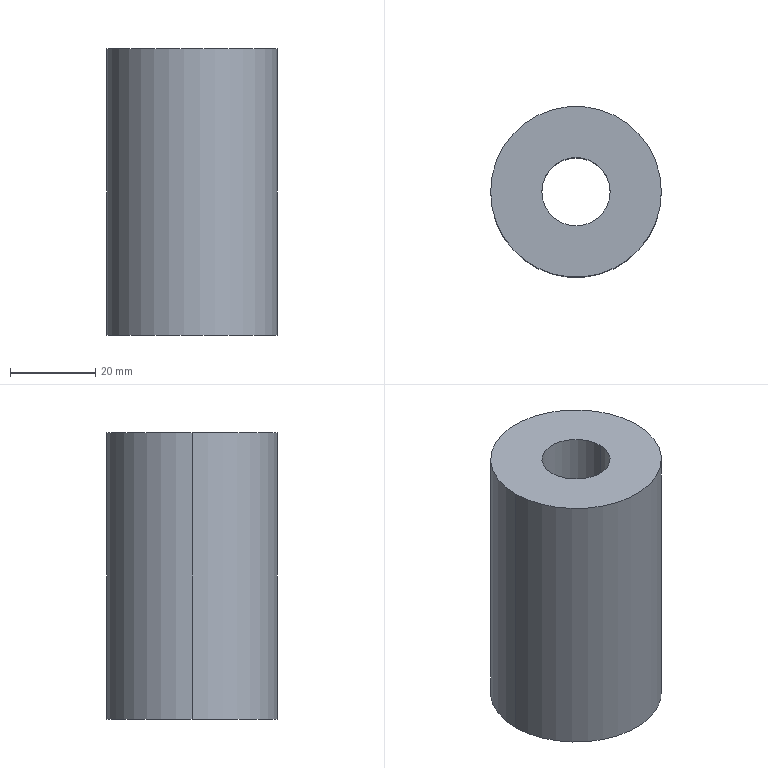Part | SolidWorks | features Extrusion 1, ICE 1 | 1 solid | 6 faces | box 40 x 40 x 67 mm | volume 70724 mm3 | cylinder 4 | plane 2 | commonest cylinder face diameters 16 x2 40 x2
STEP:
#1=CARTESIAN_POINT('',(-8.,0.,0.));
#2=VERTEX_POINT('',#1);
#3=CARTESIAN_POINT('',(8.,0.,0.));
#4=VERTEX_POINT('',#3);
#5=CARTESIAN_POINT('',(0.,0.,0.));
#6=DIRECTION('',(0.,0.,1.));
#7=DIRECTION('',(1.,0.,0.));
#8=AXIS2_PLACEMENT_3D('',#5,#6,#7);
#9=CIRCLE('',#8,8.);
#10=EDGE_CURVE('',#2,#4,#9,.T.);
#11=ORIENTED_EDGE('',*,*,#10,.F.);
#12=CARTESIAN_POINT('',(-8.,0.,67.));
#13=VERTEX_POINT('',#12);
#14=CARTESIAN_POINT('',(-8.,0.,-34.));
#15=DIRECTION('',(0.,0.,1.));
#16=VECTOR('',#15,1000.);
#17=LINE('',#14,#16);
#18=EDGE_CURVE('',#2,#13,#17,.T.);
#19=ORIENTED_EDGE('',*,*,#18,.T.);
#20=CARTESIAN_POINT('',(8.,0.,67.));
#21=VERTEX_POINT('',#20);
#22=CARTESIAN_POINT('',(0.,0.,67.));
#23=DIRECTION('',(0.,0.,1.));
#24=DIRECTION('',(1.,0.,0.));
#25=AXIS2_PLACEMENT_3D('',#22,#23,#24);
#26=CIRCLE('',#25,8.);
#27=EDGE_CURVE('',#13,#21,#26,.T.);
#28=ORIENTED_EDGE('',*,*,#27,.T.);
#29=CARTESIAN_POINT('',(8.,0.,-34.));
#30=DIRECTION('',(0.,0.,1.));
#31=VECTOR('',#30,1000.);
#32=LINE('',#29,#31);
#33=EDGE_CURVE('',#4,#21,#32,.T.);
#34=ORIENTED_EDGE('',*,*,#33,.F.);
#35=EDGE_LOOP('',(#11,#19,#28,#34));
#36=FACE_OUTER_BOUND('',#35,.T.);
#37=CARTESIAN_POINT('',(0.,0.,-34.));
#38=DIRECTION('',(0.,0.,1.));
#39=DIRECTION('',(1.,0.,0.));
#40=AXIS2_PLACEMENT_3D('',#37,#38,#39);
#41=CYLINDRICAL_SURFACE('',#40,8.);
#42=ADVANCED_FACE('',(#36),#41,.F.);
#43=CARTESIAN_POINT('',(20.,0.,67.));
#44=VERTEX_POINT('',#43);
#45=CARTESIAN_POINT('',(-20.,0.,67.));
#46=VERTEX_POINT('',#45);
#47=CARTESIAN_POINT('',(0.,0.,67.));
#48=DIRECTION('',(0.,0.,1.));
#49=DIRECTION('',(1.,0.,0.));
#50=AXIS2_PLACEMENT_3D('',#47,#48,#49);
#51=CIRCLE('',#50,20.);
#52=EDGE_CURVE('',#44,#46,#51,.T.);
#53=ORIENTED_EDGE('',*,*,#52,.F.);
#54=CARTESIAN_POINT('',(20.,0.,0.));
#55=VERTEX_POINT('',#54);
#56=CARTESIAN_POINT('',(20.,0.,67.));
#57=DIRECTION('',(0.,0.,-1.));
#58=VECTOR('',#57,1000.);
#59=LINE('',#56,#58);
#60=EDGE_CURVE('',#44,#55,#59,.T.);
#61=ORIENTED_EDGE('',*,*,#60,.T.);
#62=CARTESIAN_POINT('',(-20.,0.,0.));
#63=VERTEX_POINT('',#62);
#64=CARTESIAN_POINT('',(0.,0.,0.));
#65=DIRECTION('',(0.,0.,1.));
#66=DIRECTION('',(1.,0.,0.));
#67=AXIS2_PLACEMENT_3D('',#64,#65,#66);
#68=CIRCLE('',#67,20.);
#69=EDGE_CURVE('',#55,#63,#68,.T.);
#70=ORIENTED_EDGE('',*,*,#69,.T.);
#71=CARTESIAN_POINT('',(-20.,0.,67.));
#72=DIRECTION('',(0.,0.,-1.));
#73=VECTOR('',#72,1000.);
#74=LINE('',#71,#73);
#75=EDGE_CURVE('',#46,#63,#74,.T.);
#76=ORIENTED_EDGE('',*,*,#75,.F.);
#77=EDGE_LOOP('',(#53,#61,#70,#76));
#78=FACE_OUTER_BOUND('',#77,.T.);
#79=CARTESIAN_POINT('',(0.,0.,67.));
#80=DIRECTION('',(0.,0.,-1.));
#81=DIRECTION('',(-1.,0.,0.));
#82=AXIS2_PLACEMENT_3D('',#79,#80,#81);
#83=CYLINDRICAL_SURFACE('',#82,20.);
#84=ADVANCED_FACE('',(#78),#83,.T.);
#85=ORIENTED_EDGE('',*,*,#60,.F.);
#86=CARTESIAN_POINT('',(0.,0.,67.));
#87=DIRECTION('',(0.,0.,1.));
#88=DIRECTION('',(1.,0.,0.));
#89=AXIS2_PLACEMENT_3D('',#86,#87,#88);
#90=CIRCLE('',#89,20.);
#91=EDGE_CURVE('',#46,#44,#90,.T.);
#92=ORIENTED_EDGE('',*,*,#91,.F.);
#93=ORIENTED_EDGE('',*,*,#75,.T.);
#94=CARTESIAN_POINT('',(0.,0.,0.));
#95=DIRECTION('',(0.,0.,1.));
#96=DIRECTION('',(1.,0.,0.));
#97=AXIS2_PLACEMENT_3D('',#94,#95,#96);
#98=CIRCLE('',#97,20.);
#99=EDGE_CURVE('',#63,#55,#98,.T.);
#100=ORIENTED_EDGE('',*,*,#99,.T.);
#101=EDGE_LOOP('',(#85,#92,#93,#100));
#102=FACE_OUTER_BOUND('',#101,.T.);
#103=CARTESIAN_POINT('',(0.,0.,67.));
#104=DIRECTION('',(0.,0.,-1.));
#105=DIRECTION('',(-1.,0.,0.));
#106=AXIS2_PLACEMENT_3D('',#103,#104,#105);
#107=CYLINDRICAL_SURFACE('',#106,20.);
#108=ADVANCED_FACE('',(#102),#107,.T.);
#109=CARTESIAN_POINT('',(0.,0.,67.));
#110=DIRECTION('',(0.,0.,1.));
#111=DIRECTION('',(1.,0.,0.));
#112=AXIS2_PLACEMENT_3D('',#109,#110,#111);
#113=CIRCLE('',#112,8.);
#114=EDGE_CURVE('',#21,#13,#113,.T.);
#115=ORIENTED_EDGE('',*,*,#114,.F.);
#116=ORIENTED_EDGE('',*,*,#27,.F.);
#117=EDGE_LOOP('',(#115,#116));
#118=FACE_BOUND('',#117,.T.);
#119=ORIENTED_EDGE('',*,*,#91,.T.);
#120=ORIENTED_EDGE('',*,*,#52,.T.);
#121=EDGE_LOOP('',(#119,#120));
#122=FACE_OUTER_BOUND('',#121,.T.);
#123=CARTESIAN_POINT('',(0.,0.,67.));
#124=DIRECTION('',(0.,0.,1.));
#125=DIRECTION('',(1.,0.,0.));
#126=AXIS2_PLACEMENT_3D('',#123,#124,#125);
#127=PLANE('',#126);
#128=ADVANCED_FACE('',(#118,#122),#127,.T.);
#129=CARTESIAN_POINT('',(0.,0.,0.));
#130=DIRECTION('',(0.,0.,1.));
#131=DIRECTION('',(1.,0.,0.));
#132=AXIS2_PLACEMENT_3D('',#129,#130,#131);
#133=CIRCLE('',#132,8.);
#134=EDGE_CURVE('',#4,#2,#133,.T.);
#135=ORIENTED_EDGE('',*,*,#134,.T.);
#136=ORIENTED_EDGE('',*,*,#10,.T.);
#137=EDGE_LOOP('',(#135,#136));
#138=FACE_BOUND('',#137,.T.);
#139=ORIENTED_EDGE('',*,*,#99,.F.);
#140=ORIENTED_EDGE('',*,*,#69,.F.);
#141=EDGE_LOOP('',(#139,#140));
#142=FACE_OUTER_BOUND('',#141,.T.);
#143=CARTESIAN_POINT('',(0.,0.,0.));
#144=DIRECTION('',(0.,0.,1.));
#145=DIRECTION('',(1.,0.,0.));
#146=AXIS2_PLACEMENT_3D('',#143,#144,#145);
#147=PLANE('',#146);
#148=ADVANCED_FACE('',(#138,#142),#147,.F.);
#149=ORIENTED_EDGE('',*,*,#18,.F.);
#150=ORIENTED_EDGE('',*,*,#134,.F.);
#151=ORIENTED_EDGE('',*,*,#33,.T.);
#152=ORIENTED_EDGE('',*,*,#114,.T.);
#153=EDGE_LOOP('',(#149,#150,#151,#152));
#154=FACE_OUTER_BOUND('',#153,.T.);
#155=CARTESIAN_POINT('',(0.,0.,-34.));
#156=DIRECTION('',(0.,0.,1.));
#157=DIRECTION('',(1.,0.,0.));
#158=AXIS2_PLACEMENT_3D('',#155,#156,#157);
#159=CYLINDRICAL_SURFACE('',#158,8.);
#160=ADVANCED_FACE('',(#154),#159,.F.);
#161=CLOSED_SHELL('',(#42,#84,#108,#128,#148,#160));
#162=MANIFOLD_SOLID_BREP('',#161);
#163=CARTESIAN_POINT('',(0.,0.,0.));
#164=DIRECTION('',(0.,0.,1.));
#165=DIRECTION('',(1.,0.,0.));
#166=AXIS2_PLACEMENT_3D('',#163,#164,#165);
#167=(LENGTH_UNIT()NAMED_UNIT(*)SI_UNIT(.MILLI.,.METRE.));
#168=UNCERTAINTY_MEASURE_WITH_UNIT(LENGTH_MEASURE(0.00001),#167,'','');
#169=(NAMED_UNIT(*)PLANE_ANGLE_UNIT()SI_UNIT($,.RADIAN.));
#170=(NAMED_UNIT(*)SI_UNIT($,.STERADIAN.)SOLID_ANGLE_UNIT());
#171=(GEOMETRIC_REPRESENTATION_CONTEXT(3)GLOBAL_UNCERTAINTY_ASSIGNED_CONTEXT((#168))GLOBAL_UNIT_ASSIGNED_CONTEXT((#167,#169,#170))REPRESENTATION_CONTEXT('',''));
#172=ADVANCED_BREP_SHAPE_REPRESENTATION('',(#162,#166),#171);